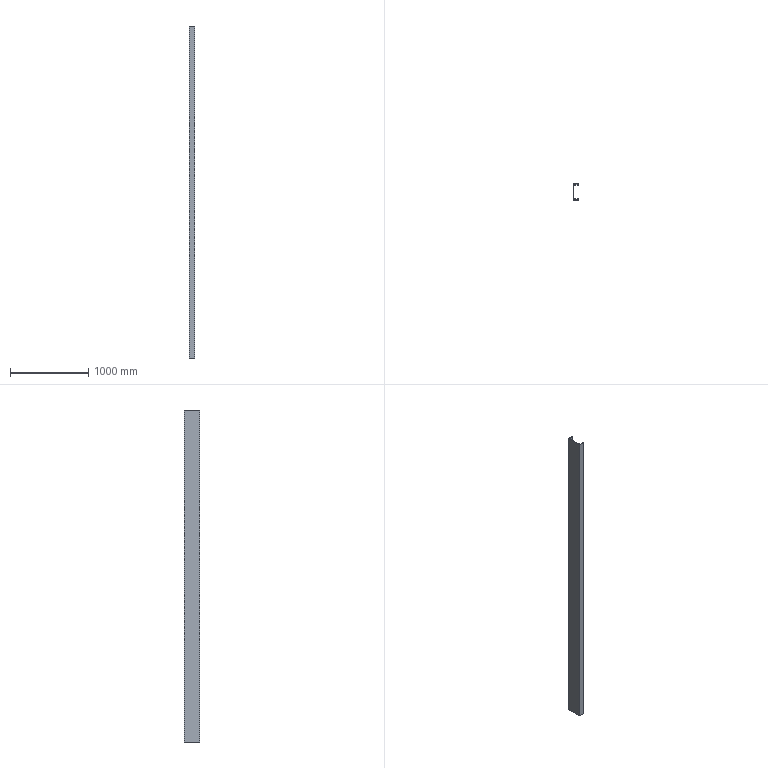Part | SolidWorks | features Extrusion 1 | 1 solid | 14 faces | box 73 x 200 x 4242 mm | volume 12148294 mm3 | plane 10 | cylinder 4 | commonest cylinder face diameters 11 x2 22 x2
STEP:
#1=CARTESIAN_POINT('',(73.,200.,-2120.9));
#2=VERTEX_POINT('',#1);
#3=CARTESIAN_POINT('',(0.,200.,-2120.9));
#4=VERTEX_POINT('',#3);
#5=CARTESIAN_POINT('',(0.,200.,-2120.9));
#6=DIRECTION('',(-1.,0.,0.));
#7=VECTOR('',#6,1000.);
#8=LINE('',#5,#7);
#9=EDGE_CURVE('',#2,#4,#8,.T.);
#10=ORIENTED_EDGE('',*,*,#9,.T.);
#11=CARTESIAN_POINT('',(0.,200.,2120.9));
#12=VERTEX_POINT('',#11);
#13=CARTESIAN_POINT('',(0.,200.,2120.9));
#14=DIRECTION('',(0.,0.,-1.));
#15=VECTOR('',#14,1000.);
#16=LINE('',#13,#15);
#17=EDGE_CURVE('',#12,#4,#16,.T.);
#18=ORIENTED_EDGE('',*,*,#17,.F.);
#19=CARTESIAN_POINT('',(73.,200.,2120.9));
#20=VERTEX_POINT('',#19);
#21=CARTESIAN_POINT('',(0.,200.,2120.9));
#22=DIRECTION('',(-1.,0.,0.));
#23=VECTOR('',#22,1000.);
#24=LINE('',#21,#23);
#25=EDGE_CURVE('',#20,#12,#24,.T.);
#26=ORIENTED_EDGE('',*,*,#25,.F.);
#27=CARTESIAN_POINT('',(73.,200.,2120.9));
#28=DIRECTION('',(0.,0.,-1.));
#29=VECTOR('',#28,1000.);
#30=LINE('',#27,#29);
#31=EDGE_CURVE('',#20,#2,#30,.T.);
#32=ORIENTED_EDGE('',*,*,#31,.T.);
#33=EDGE_LOOP('',(#10,#18,#26,#32));
#34=FACE_OUTER_BOUND('',#33,.T.);
#35=CARTESIAN_POINT('',(0.,200.,2120.9));
#36=DIRECTION('',(0.,-1.,0.));
#37=DIRECTION('',(0.,0.,-1.));
#38=AXIS2_PLACEMENT_3D('',#35,#36,#37);
#39=PLANE('',#38);
#40=ADVANCED_FACE('',(#34),#39,.F.);
#41=CARTESIAN_POINT('',(0.,0.,-2120.9));
#42=VERTEX_POINT('',#41);
#43=CARTESIAN_POINT('',(0.,0.,-2120.9));
#44=DIRECTION('',(0.,-1.,0.));
#45=VECTOR('',#44,1000.);
#46=LINE('',#43,#45);
#47=EDGE_CURVE('',#4,#42,#46,.T.);
#48=ORIENTED_EDGE('',*,*,#47,.T.);
#49=CARTESIAN_POINT('',(0.,0.,2120.9));
#50=VERTEX_POINT('',#49);
#51=CARTESIAN_POINT('',(0.,0.,2120.9));
#52=DIRECTION('',(0.,0.,-1.));
#53=VECTOR('',#52,1000.);
#54=LINE('',#51,#53);
#55=EDGE_CURVE('',#50,#42,#54,.T.);
#56=ORIENTED_EDGE('',*,*,#55,.F.);
#57=CARTESIAN_POINT('',(0.,0.,2120.9));
#58=DIRECTION('',(0.,-1.,0.));
#59=VECTOR('',#58,1000.);
#60=LINE('',#57,#59);
#61=EDGE_CURVE('',#12,#50,#60,.T.);
#62=ORIENTED_EDGE('',*,*,#61,.F.);
#63=ORIENTED_EDGE('',*,*,#17,.T.);
#64=EDGE_LOOP('',(#48,#56,#62,#63));
#65=FACE_OUTER_BOUND('',#64,.T.);
#66=CARTESIAN_POINT('',(0.,0.,2120.9));
#67=DIRECTION('',(1.,0.,0.));
#68=DIRECTION('',(0.,0.,-1.));
#69=AXIS2_PLACEMENT_3D('',#66,#67,#68);
#70=PLANE('',#69);
#71=ADVANCED_FACE('',(#65),#70,.F.);
#72=CARTESIAN_POINT('',(73.,0.,-2120.9));
#73=VERTEX_POINT('',#72);
#74=CARTESIAN_POINT('',(0.,0.,-2120.9));
#75=DIRECTION('',(1.,0.,0.));
#76=VECTOR('',#75,1000.);
#77=LINE('',#74,#76);
#78=EDGE_CURVE('',#42,#73,#77,.T.);
#79=ORIENTED_EDGE('',*,*,#78,.T.);
#80=CARTESIAN_POINT('',(73.,0.,2120.9));
#81=VERTEX_POINT('',#80);
#82=CARTESIAN_POINT('',(73.,0.,2120.9));
#83=DIRECTION('',(0.,0.,-1.));
#84=VECTOR('',#83,1000.);
#85=LINE('',#82,#84);
#86=EDGE_CURVE('',#81,#73,#85,.T.);
#87=ORIENTED_EDGE('',*,*,#86,.F.);
#88=CARTESIAN_POINT('',(0.,0.,2120.9));
#89=DIRECTION('',(1.,0.,0.));
#90=VECTOR('',#89,1000.);
#91=LINE('',#88,#90);
#92=EDGE_CURVE('',#50,#81,#91,.T.);
#93=ORIENTED_EDGE('',*,*,#92,.F.);
#94=ORIENTED_EDGE('',*,*,#55,.T.);
#95=EDGE_LOOP('',(#79,#87,#93,#94));
#96=FACE_OUTER_BOUND('',#95,.T.);
#97=CARTESIAN_POINT('',(0.,0.,2120.9));
#98=DIRECTION('',(0.,1.,0.));
#99=DIRECTION('',(0.,0.,1.));
#100=AXIS2_PLACEMENT_3D('',#97,#98,#99);
#101=PLANE('',#100);
#102=ADVANCED_FACE('',(#96),#101,.F.);
#103=CARTESIAN_POINT('',(73.,3.967,-2120.9));
#104=VERTEX_POINT('',#103);
#105=CARTESIAN_POINT('',(73.,3.967,-2120.9));
#106=DIRECTION('',(0.,1.,0.));
#107=VECTOR('',#106,1000.);
#108=LINE('',#105,#107);
#109=EDGE_CURVE('',#73,#104,#108,.T.);
#110=ORIENTED_EDGE('',*,*,#109,.T.);
#111=CARTESIAN_POINT('',(73.,3.967,2120.9));
#112=VERTEX_POINT('',#111);
#113=CARTESIAN_POINT('',(73.,3.967,2120.9));
#114=DIRECTION('',(0.,0.,-1.));
#115=VECTOR('',#114,1000.);
#116=LINE('',#113,#115);
#117=EDGE_CURVE('',#112,#104,#116,.T.);
#118=ORIENTED_EDGE('',*,*,#117,.F.);
#119=CARTESIAN_POINT('',(73.,3.967,2120.9));
#120=DIRECTION('',(0.,1.,0.));
#121=VECTOR('',#120,1000.);
#122=LINE('',#119,#121);
#123=EDGE_CURVE('',#81,#112,#122,.T.);
#124=ORIENTED_EDGE('',*,*,#123,.F.);
#125=ORIENTED_EDGE('',*,*,#86,.T.);
#126=EDGE_LOOP('',(#110,#118,#124,#125));
#127=FACE_OUTER_BOUND('',#126,.T.);
#128=CARTESIAN_POINT('',(73.,3.967,2120.9));
#129=DIRECTION('',(-1.,0.,0.));
#130=DIRECTION('',(0.,-1.,0.));
#131=AXIS2_PLACEMENT_3D('',#128,#129,#130);
#132=PLANE('',#131);
#133=ADVANCED_FACE('',(#127),#132,.F.);
#134=CARTESIAN_POINT('',(67.771,9.46,-2120.9));
#135=VERTEX_POINT('',#134);
#136=CARTESIAN_POINT('',(67.5,3.967,-2120.9));
#137=DIRECTION('',(0.,0.,1.));
#138=DIRECTION('',(1.,0.,0.));
#139=AXIS2_PLACEMENT_3D('',#136,#137,#138);
#140=CIRCLE('',#139,5.5);
#141=EDGE_CURVE('',#104,#135,#140,.T.);
#142=ORIENTED_EDGE('',*,*,#141,.T.);
#143=CARTESIAN_POINT('',(67.771,9.46,2120.9));
#144=VERTEX_POINT('',#143);
#145=CARTESIAN_POINT('',(67.771,9.46,2120.9));
#146=DIRECTION('',(0.,0.,-1.));
#147=VECTOR('',#146,1000.);
#148=LINE('',#145,#147);
#149=EDGE_CURVE('',#144,#135,#148,.T.);
#150=ORIENTED_EDGE('',*,*,#149,.F.);
#151=CARTESIAN_POINT('',(67.5,3.967,2120.9));
#152=DIRECTION('',(0.,0.,1.));
#153=DIRECTION('',(1.,0.,0.));
#154=AXIS2_PLACEMENT_3D('',#151,#152,#153);
#155=CIRCLE('',#154,5.5);
#156=EDGE_CURVE('',#112,#144,#155,.T.);
#157=ORIENTED_EDGE('',*,*,#156,.F.);
#158=ORIENTED_EDGE('',*,*,#117,.T.);
#159=EDGE_LOOP('',(#142,#150,#157,#158));
#160=FACE_OUTER_BOUND('',#159,.T.);
#161=CARTESIAN_POINT('',(67.5,3.967,2120.9));
#162=DIRECTION('',(0.,0.,-1.));
#163=DIRECTION('',(-1.,0.,0.));
#164=AXIS2_PLACEMENT_3D('',#161,#162,#163);
#165=CYLINDRICAL_SURFACE('',#164,5.5);
#166=ADVANCED_FACE('',(#160),#165,.T.);
#167=CARTESIAN_POINT('',(17.459,11.938,-2120.9));
#168=VERTEX_POINT('',#167);
#169=CARTESIAN_POINT('',(17.459,11.938,-2120.9));
#170=DIRECTION('',(-0.9988,0.04918,0.));
#171=VECTOR('',#170,1000.);
#172=LINE('',#169,#171);
#173=EDGE_CURVE('',#135,#168,#172,.T.);
#174=ORIENTED_EDGE('',*,*,#173,.T.);
#175=CARTESIAN_POINT('',(17.459,11.938,2120.9));
#176=VERTEX_POINT('',#175);
#177=CARTESIAN_POINT('',(17.459,11.938,2120.9));
#178=DIRECTION('',(0.,0.,-1.));
#179=VECTOR('',#178,1000.);
#180=LINE('',#177,#179);
#181=EDGE_CURVE('',#176,#168,#180,.T.);
#182=ORIENTED_EDGE('',*,*,#181,.F.);
#183=CARTESIAN_POINT('',(17.459,11.938,2120.9));
#184=DIRECTION('',(-0.9988,0.04918,0.));
#185=VECTOR('',#184,1000.);
#186=LINE('',#183,#185);
#187=EDGE_CURVE('',#144,#176,#186,.T.);
#188=ORIENTED_EDGE('',*,*,#187,.F.);
#189=ORIENTED_EDGE('',*,*,#149,.T.);
#190=EDGE_LOOP('',(#174,#182,#188,#189));
#191=FACE_OUTER_BOUND('',#190,.T.);
#192=CARTESIAN_POINT('',(17.459,11.938,2120.9));
#193=DIRECTION('',(-0.04918,-0.9988,0.));
#194=DIRECTION('',(0.9988,-0.04918,0.));
#195=AXIS2_PLACEMENT_3D('',#192,#193,#194);
#196=PLANE('',#195);
#197=ADVANCED_FACE('',(#191),#196,.F.);
#198=CARTESIAN_POINT('',(7.,22.924,-2120.9));
#199=VERTEX_POINT('',#198);
#200=CARTESIAN_POINT('',(18.,22.924,-2120.9));
#201=DIRECTION('',(0.,0.,-1.));
#202=DIRECTION('',(-1.,0.,0.));
#203=AXIS2_PLACEMENT_3D('',#200,#201,#202);
#204=CIRCLE('',#203,11.);
#205=EDGE_CURVE('',#168,#199,#204,.T.);
#206=ORIENTED_EDGE('',*,*,#205,.T.);
#207=CARTESIAN_POINT('',(7.,22.924,2120.9));
#208=VERTEX_POINT('',#207);
#209=CARTESIAN_POINT('',(7.,22.924,2120.9));
#210=DIRECTION('',(0.,0.,-1.));
#211=VECTOR('',#210,1000.);
#212=LINE('',#209,#211);
#213=EDGE_CURVE('',#208,#199,#212,.T.);
#214=ORIENTED_EDGE('',*,*,#213,.F.);
#215=CARTESIAN_POINT('',(18.,22.924,2120.9));
#216=DIRECTION('',(0.,0.,-1.));
#217=DIRECTION('',(-1.,0.,0.));
#218=AXIS2_PLACEMENT_3D('',#215,#216,#217);
#219=CIRCLE('',#218,11.);
#220=EDGE_CURVE('',#176,#208,#219,.T.);
#221=ORIENTED_EDGE('',*,*,#220,.F.);
#222=ORIENTED_EDGE('',*,*,#181,.T.);
#223=EDGE_LOOP('',(#206,#214,#221,#222));
#224=FACE_OUTER_BOUND('',#223,.T.);
#225=CARTESIAN_POINT('',(18.,22.924,2120.9));
#226=DIRECTION('',(0.,0.,-1.));
#227=DIRECTION('',(-1.,0.,0.));
#228=AXIS2_PLACEMENT_3D('',#225,#226,#227);
#229=CYLINDRICAL_SURFACE('',#228,11.);
#230=ADVANCED_FACE('',(#224),#229,.F.);
#231=CARTESIAN_POINT('',(7.,177.076,-2120.9));
#232=VERTEX_POINT('',#231);
#233=CARTESIAN_POINT('',(7.,177.076,-2120.9));
#234=DIRECTION('',(0.,1.,0.));
#235=VECTOR('',#234,1000.);
#236=LINE('',#233,#235);
#237=EDGE_CURVE('',#199,#232,#236,.T.);
#238=ORIENTED_EDGE('',*,*,#237,.T.);
#239=CARTESIAN_POINT('',(7.,177.076,2120.9));
#240=VERTEX_POINT('',#239);
#241=CARTESIAN_POINT('',(7.,177.076,2120.9));
#242=DIRECTION('',(0.,0.,-1.));
#243=VECTOR('',#242,1000.);
#244=LINE('',#241,#243);
#245=EDGE_CURVE('',#240,#232,#244,.T.);
#246=ORIENTED_EDGE('',*,*,#245,.F.);
#247=CARTESIAN_POINT('',(7.,177.076,2120.9));
#248=DIRECTION('',(0.,1.,0.));
#249=VECTOR('',#248,1000.);
#250=LINE('',#247,#249);
#251=EDGE_CURVE('',#208,#240,#250,.T.);
#252=ORIENTED_EDGE('',*,*,#251,.F.);
#253=ORIENTED_EDGE('',*,*,#213,.T.);
#254=EDGE_LOOP('',(#238,#246,#252,#253));
#255=FACE_OUTER_BOUND('',#254,.T.);
#256=CARTESIAN_POINT('',(7.,177.076,2120.9));
#257=DIRECTION('',(-1.,0.,0.));
#258=DIRECTION('',(0.,0.,1.));
#259=AXIS2_PLACEMENT_3D('',#256,#257,#258);
#260=PLANE('',#259);
#261=ADVANCED_FACE('',(#255),#260,.F.);
#262=CARTESIAN_POINT('',(17.459,188.062,-2120.9));
#263=VERTEX_POINT('',#262);
#264=CARTESIAN_POINT('',(18.,177.076,-2120.9));
#265=DIRECTION('',(0.,0.,-1.));
#266=DIRECTION('',(-1.,0.,0.));
#267=AXIS2_PLACEMENT_3D('',#264,#265,#266);
#268=CIRCLE('',#267,11.);
#269=EDGE_CURVE('',#232,#263,#268,.T.);
#270=ORIENTED_EDGE('',*,*,#269,.T.);
#271=CARTESIAN_POINT('',(17.459,188.062,2120.9));
#272=VERTEX_POINT('',#271);
#273=CARTESIAN_POINT('',(17.459,188.062,2120.9));
#274=DIRECTION('',(0.,0.,-1.));
#275=VECTOR('',#274,1000.);
#276=LINE('',#273,#275);
#277=EDGE_CURVE('',#272,#263,#276,.T.);
#278=ORIENTED_EDGE('',*,*,#277,.F.);
#279=CARTESIAN_POINT('',(18.,177.076,2120.9));
#280=DIRECTION('',(0.,0.,-1.));
#281=DIRECTION('',(-1.,0.,0.));
#282=AXIS2_PLACEMENT_3D('',#279,#280,#281);
#283=CIRCLE('',#282,11.);
#284=EDGE_CURVE('',#240,#272,#283,.T.);
#285=ORIENTED_EDGE('',*,*,#284,.F.);
#286=ORIENTED_EDGE('',*,*,#245,.T.);
#287=EDGE_LOOP('',(#270,#278,#285,#286));
#288=FACE_OUTER_BOUND('',#287,.T.);
#289=CARTESIAN_POINT('',(18.,177.076,2120.9));
#290=DIRECTION('',(0.,0.,-1.));
#291=DIRECTION('',(-1.,0.,0.));
#292=AXIS2_PLACEMENT_3D('',#289,#290,#291);
#293=CYLINDRICAL_SURFACE('',#292,11.);
#294=ADVANCED_FACE('',(#288),#293,.F.);
#295=CARTESIAN_POINT('',(67.771,190.54,-2120.9));
#296=VERTEX_POINT('',#295);
#297=CARTESIAN_POINT('',(17.459,188.062,-2120.9));
#298=DIRECTION('',(0.9988,0.04918,0.));
#299=VECTOR('',#298,1000.);
#300=LINE('',#297,#299);
#301=EDGE_CURVE('',#263,#296,#300,.T.);
#302=ORIENTED_EDGE('',*,*,#301,.T.);
#303=CARTESIAN_POINT('',(67.771,190.54,2120.9));
#304=VERTEX_POINT('',#303);
#305=CARTESIAN_POINT('',(67.771,190.54,2120.9));
#306=DIRECTION('',(0.,0.,-1.));
#307=VECTOR('',#306,1000.);
#308=LINE('',#305,#307);
#309=EDGE_CURVE('',#304,#296,#308,.T.);
#310=ORIENTED_EDGE('',*,*,#309,.F.);
#311=CARTESIAN_POINT('',(17.459,188.062,2120.9));
#312=DIRECTION('',(0.9988,0.04918,0.));
#313=VECTOR('',#312,1000.);
#314=LINE('',#311,#313);
#315=EDGE_CURVE('',#272,#304,#314,.T.);
#316=ORIENTED_EDGE('',*,*,#315,.F.);
#317=ORIENTED_EDGE('',*,*,#277,.T.);
#318=EDGE_LOOP('',(#302,#310,#316,#317));
#319=FACE_OUTER_BOUND('',#318,.T.);
#320=CARTESIAN_POINT('',(17.459,188.062,2120.9));
#321=DIRECTION('',(-0.04918,0.9988,0.));
#322=DIRECTION('',(-0.9988,-0.04918,0.));
#323=AXIS2_PLACEMENT_3D('',#320,#321,#322);
#324=PLANE('',#323);
#325=ADVANCED_FACE('',(#319),#324,.F.);
#326=CARTESIAN_POINT('',(73.,196.033,-2120.9));
#327=VERTEX_POINT('',#326);
#328=CARTESIAN_POINT('',(67.5,196.033,-2120.9));
#329=DIRECTION('',(0.,0.,1.));
#330=DIRECTION('',(1.,0.,0.));
#331=AXIS2_PLACEMENT_3D('',#328,#329,#330);
#332=CIRCLE('',#331,5.5);
#333=EDGE_CURVE('',#296,#327,#332,.T.);
#334=ORIENTED_EDGE('',*,*,#333,.T.);
#335=CARTESIAN_POINT('',(73.,196.033,2120.9));
#336=VERTEX_POINT('',#335);
#337=CARTESIAN_POINT('',(73.,196.033,2120.9));
#338=DIRECTION('',(0.,0.,-1.));
#339=VECTOR('',#338,1000.);
#340=LINE('',#337,#339);
#341=EDGE_CURVE('',#336,#327,#340,.T.);
#342=ORIENTED_EDGE('',*,*,#341,.F.);
#343=CARTESIAN_POINT('',(67.5,196.033,2120.9));
#344=DIRECTION('',(0.,0.,1.));
#345=DIRECTION('',(1.,0.,0.));
#346=AXIS2_PLACEMENT_3D('',#343,#344,#345);
#347=CIRCLE('',#346,5.5);
#348=EDGE_CURVE('',#304,#336,#347,.T.);
#349=ORIENTED_EDGE('',*,*,#348,.F.);
#350=ORIENTED_EDGE('',*,*,#309,.T.);
#351=EDGE_LOOP('',(#334,#342,#349,#350));
#352=FACE_OUTER_BOUND('',#351,.T.);
#353=CARTESIAN_POINT('',(67.5,196.033,2120.9));
#354=DIRECTION('',(0.,0.,-1.));
#355=DIRECTION('',(-1.,0.,0.));
#356=AXIS2_PLACEMENT_3D('',#353,#354,#355);
#357=CYLINDRICAL_SURFACE('',#356,5.5);
#358=ADVANCED_FACE('',(#352),#357,.T.);
#359=CARTESIAN_POINT('',(73.,196.033,-2120.9));
#360=DIRECTION('',(0.,1.,0.));
#361=VECTOR('',#360,1000.);
#362=LINE('',#359,#361);
#363=EDGE_CURVE('',#327,#2,#362,.T.);
#364=ORIENTED_EDGE('',*,*,#363,.T.);
#365=ORIENTED_EDGE('',*,*,#31,.F.);
#366=CARTESIAN_POINT('',(73.,196.033,2120.9));
#367=DIRECTION('',(0.,1.,0.));
#368=VECTOR('',#367,1000.);
#369=LINE('',#366,#368);
#370=EDGE_CURVE('',#336,#20,#369,.T.);
#371=ORIENTED_EDGE('',*,*,#370,.F.);
#372=ORIENTED_EDGE('',*,*,#341,.T.);
#373=EDGE_LOOP('',(#364,#365,#371,#372));
#374=FACE_OUTER_BOUND('',#373,.T.);
#375=CARTESIAN_POINT('',(73.,196.033,2120.9));
#376=DIRECTION('',(-1.,0.,0.));
#377=DIRECTION('',(0.,-1.,0.));
#378=AXIS2_PLACEMENT_3D('',#375,#376,#377);
#379=PLANE('',#378);
#380=ADVANCED_FACE('',(#374),#379,.F.);
#381=ORIENTED_EDGE('',*,*,#25,.T.);
#382=ORIENTED_EDGE('',*,*,#61,.T.);
#383=ORIENTED_EDGE('',*,*,#92,.T.);
#384=ORIENTED_EDGE('',*,*,#123,.T.);
#385=ORIENTED_EDGE('',*,*,#156,.T.);
#386=ORIENTED_EDGE('',*,*,#187,.T.);
#387=ORIENTED_EDGE('',*,*,#220,.T.);
#388=ORIENTED_EDGE('',*,*,#251,.T.);
#389=ORIENTED_EDGE('',*,*,#284,.T.);
#390=ORIENTED_EDGE('',*,*,#315,.T.);
#391=ORIENTED_EDGE('',*,*,#348,.T.);
#392=ORIENTED_EDGE('',*,*,#370,.T.);
#393=EDGE_LOOP('',(#381,#382,#383,#384,#385,#386,#387,#388,#389,#390,#391,#392));
#394=FACE_OUTER_BOUND('',#393,.T.);
#395=CARTESIAN_POINT('',(67.5,196.033,2120.9));
#396=DIRECTION('',(0.,0.,1.));
#397=DIRECTION('',(1.,0.,0.));
#398=AXIS2_PLACEMENT_3D('',#395,#396,#397);
#399=PLANE('',#398);
#400=ADVANCED_FACE('',(#394),#399,.T.);
#401=ORIENTED_EDGE('',*,*,#9,.F.);
#402=ORIENTED_EDGE('',*,*,#363,.F.);
#403=ORIENTED_EDGE('',*,*,#333,.F.);
#404=ORIENTED_EDGE('',*,*,#301,.F.);
#405=ORIENTED_EDGE('',*,*,#269,.F.);
#406=ORIENTED_EDGE('',*,*,#237,.F.);
#407=ORIENTED_EDGE('',*,*,#205,.F.);
#408=ORIENTED_EDGE('',*,*,#173,.F.);
#409=ORIENTED_EDGE('',*,*,#141,.F.);
#410=ORIENTED_EDGE('',*,*,#109,.F.);
#411=ORIENTED_EDGE('',*,*,#78,.F.);
#412=ORIENTED_EDGE('',*,*,#47,.F.);
#413=EDGE_LOOP('',(#401,#402,#403,#404,#405,#406,#407,#408,#409,#410,#411,#412));
#414=FACE_OUTER_BOUND('',#413,.T.);
#415=CARTESIAN_POINT('',(67.5,196.033,-2120.9));
#416=DIRECTION('',(0.,0.,1.));
#417=DIRECTION('',(1.,0.,0.));
#418=AXIS2_PLACEMENT_3D('',#415,#416,#417);
#419=PLANE('',#418);
#420=ADVANCED_FACE('',(#414),#419,.F.);
#421=CLOSED_SHELL('',(#40,#71,#102,#133,#166,#197,#230,#261,#294,#325,#358,#380,#400,#420));
#422=MANIFOLD_SOLID_BREP('',#421);
#423=CARTESIAN_POINT('',(0.,0.,0.));
#424=DIRECTION('',(0.,0.,1.));
#425=DIRECTION('',(1.,0.,0.));
#426=AXIS2_PLACEMENT_3D('',#423,#424,#425);
#427=(LENGTH_UNIT()NAMED_UNIT(*)SI_UNIT(.MILLI.,.METRE.));
#428=UNCERTAINTY_MEASURE_WITH_UNIT(LENGTH_MEASURE(0.00001),#427,'','');
#429=(NAMED_UNIT(*)PLANE_ANGLE_UNIT()SI_UNIT($,.RADIAN.));
#430=(NAMED_UNIT(*)SI_UNIT($,.STERADIAN.)SOLID_ANGLE_UNIT());
#431=(GEOMETRIC_REPRESENTATION_CONTEXT(3)GLOBAL_UNCERTAINTY_ASSIGNED_CONTEXT((#428))GLOBAL_UNIT_ASSIGNED_CONTEXT((#427,#429,#430))REPRESENTATION_CONTEXT('',''));
#432=ADVANCED_BREP_SHAPE_REPRESENTATION('',(#422,#426),#431);